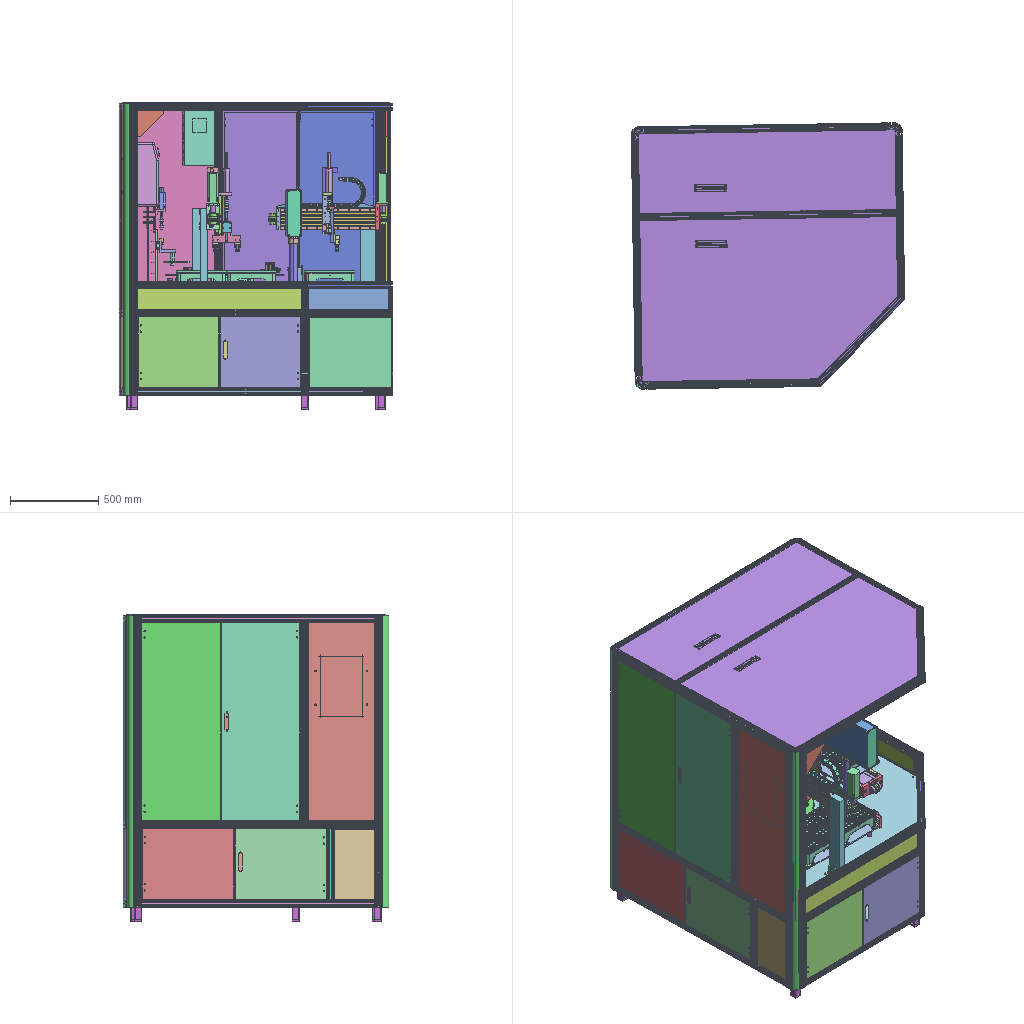Assembly | SolidWorks | 176 different items | 401 placed | box 1545 x 1502 x 1731 mm
Parts list (item | name | quantity | parent item):
1 | 12X20带轮  | x8 | in 25, 41, 57, 58
2 | 15x15×495导轨700 | x2 | in 69
3 | 15×15×186.5导轨 | x2 | in 25, 41
4 | 15×15×540导轨 | x4 | in 25, 41
5 | 4040角件 | x9 | in 25, 41, 91
6 | 4080型材 | x4 | in 25, 41
7 | 40X120型材 | x2 | in 25, 41
8 | 40X160型材 | x2 | in 57, 58
9 | 40×40×170型材(默认_按加工_) | x2 | in 10, 11
10 | 40×40×170型材（附端盖）-1 (subassembly) | x1 | in 82
11 | 40×40×170型材（附端盖） (subassembly) | x1 | in 82
12 | 40×40×250型材(默认_按加工_) | x1 | in 91
13 | 40型材端盖ARC52-4010-H4040 | x5 | in 10, 11, 91
14 | 80DF+0.55KW普通电机+050减速机(2018-5-28) (subassembly) | x1 | in 21
15 | 80x40×910铝型材 | x1 | in 69
16 | CDM2B20-100Z-XC8B双杆双作用气缸 | x2 | in 25, 41
17 | DNCJ 32X35-20-PPV-A气缸 | x1 | in 69
18 | DNCJ 32X60-20-PPV-A气缸 | x1 | in 69
19 | ECMA-C20604RS带刹车带油封 | x2 | in 25, 41
20 | HL-A-KDFJ-01 机架组件 (subassembly) | x1 | -
21 | HL-A-KDFJ-02 工作台机构 (subassembly) | x1 | -
22 | HL-A-KDFJ-02.1 圆盘 | x1 | in 21
23 | HL-A-KDFJ-02.2 分割器位置检测开关固定架 | x1 | in 21
24 | HL-A-KDFJ-02.3-1 分割器位置检测开关支架(Default) | x1 | in 21
25 | HL-A-KDFJ-03 抓取机构1 (subassembly) | x1 | -
26 | HL-A-KDFJ-03.1-1 带轮固定板 | x1 | in 25
27 | HL-A-KDFJ-03.1-2 带轮固定板2 | x1 | in 25
28 | HL-A-KDFJ-03.2-1 夹爪 | x4 | in 25
29 | HL-A-KDFJ-03.2-2 夹爪橡胶套 | x4 | in 25
30 | HL-A-KDFJ-03.2-3 气缸固定架 | x1 | in 25
31 | HL-A-KDFJ-03.2-4 抓取部件 | x1 | in 25
32 | HL-A-KDFJ-03.2-5 抓取部件1 | x1 | in 25
33 | HL-A-KDFJ-03.2-6 导轨固定架 | x1 | in 25
34 | HL-A-KDFJ-03.3-1.1 12×65轴 | x1 | in 25
35 | HL-A-KDFJ-03.3-1.1 12×80轴 | x1 | in 25
36 | HL-A-KDFJ-03.4-1 卸料链支架(默认) | x1 | in 25
37 | HL-A-KDFJ-03.4-2 拖链放置架 | x1 | in 25
38 | HL-A-KDFJ-03.5-1 导向块 | x1 | in 25
39 | HL-A-KDFJ-03.5-2 固定块 | x1 | in 25
40 | HL-A-KDFJ-03.6 压皮带块 | x2 | in 25
41 | HL-A-KDFJ-04 抓取机构2 (subassembly) | x1 | -
42 | HL-A-KDFJ-04.1 带轮固定板1 | x1 | in 41
43 | HL-A-KDFJ-04.2 带轮固定板2 | x1 | in 41
44 | HL-A-KDFJ-04.2-1 夹爪 | x4 | in 41
45 | HL-A-KDFJ-04.2-2 夹爪橡胶套 | x4 | in 41
46 | HL-A-KDFJ-04.2-3 气缸固定架 | x1 | in 41
47 | HL-A-KDFJ-04.2-4 抓取部件 | x1 | in 41
48 | HL-A-KDFJ-04.2-5 抓取部件1 | x1 | in 41
49 | HL-A-KDFJ-04.2-6 导轨固定架 | x1 | in 41
50 | HL-A-KDFJ-04.3-1.1 12×65轴  | x1 | in 41
51 | HL-A-KDFJ-04.3-1.1 12×80轴  | x1 | in 41
52 | HL-A-KDFJ-04.4-1 拖链放置架 | x1 | in 41
53 | HL-A-KDFJ-04.4-2 卸料链支架2(默认) | x1 | in 41
54 | HL-A-KDFJ-04.5-1 导向块 | x1 | in 41
55 | HL-A-KDFJ-04.5-2 固定块 | x1 | in 41
56 | HL-A-KDFJ-04.6 压皮带块 | x2 | in 41
57 | HL-A-KDFJ-05 直线模组装配-1 (subassembly) | x1 | -
58 | HL-A-KDFJ-05 直线模组装配 (subassembly) | x1 | -
59 | HL-A-KDFJ-05.1-1 带轮固定板 | x2 | in 57, 58
60 | HL-A-KDFJ-05.1-2 带轮固定板1 | x2 | in 57, 58
61 | HL-A-KDFJ-05.1-3 运动板 | x2 | in 57, 58
62 | HL-A-KDFJ-05.1-4 限位块 | x8 | in 57, 58
63 | HL-A-KDFJ-05.1-5 支撑柱 | x8 | in 57, 58
64 | HL-A-KDFJ-05.1-6 限位块2 | x4 | in 57, 58
65 | HL-A-KDFJ-05.2-1.1 12×65轴 (1) | x2 | in 57, 58
66 | HL-A-KDFJ-05.2-1.2 12×80轴 (2) | x2 | in 57, 58
67 | HL-A-KDFJ-05.3-1 压皮带块 | x4 | in 57, 58
68 | HL-A-KDFJ-05.3-2 带轮压紧块 | x2 | in 57, 58
69 | HL-A-KDFJ-06 检测跳火工装 (subassembly) | x1 | -
70 | HL-A-KDFJ-06.2-1 滑块支座 | x2 | in 69
71 | HL-A-KDFJ-06.2-2 尼龙棒 | x2 | in 69
72 | HL-A-KDFJ-06.2-3 气缸垫块 | x2 | in 69
73 | HL-A-KDFJ-06.2-4 油槽托架 | x2 | in 69
74 | HL-A-KDFJ-06.2-5 支撑架1 | x1 | in 69
75 | HL-A-KDFJ-06.2-6 支撑架 | x1 | in 69
76 | HL-A-KDFJ-06.3-1 电极头 | x8 | in 69
77 | HL-A-KDFJ-06.3-2 80针 | x8 | in 69
78 | HL-A-KDFJ-06.3-3 电极座 | x8 | in 69
79 | HL-A-KDFJ-06.3-4电极头触点 | x2 | in 69
80 | HL-A-KDFJ-06.5 三针绝缘板 | x1 | in 69
81 | HL-A-KDFJ-06.6 油杯 | x4 | in 69
82 | HL-A-KDFJ-07 高压包电柜组件 (subassembly) | x1 | -
83 | HL-A-KDFJ-07.1 高压包电柜 (subassembly) | x1 | in 82
84 | HL-A-KDFJ-07.1-1 包电柜右门(默认) | x1 | in 83
85 | HL-A-KDFJ-07.1-2 包电柜左门(默认) | x1 | in 83
86 | HL-A-KDFJ-07.1-3 包电柜柜体(默认) | x1 | in 83
87 | HL-A-KDFJ-08 吹气组件 (subassembly) | x1 | -
88 | HL-A-KDFJ-08.1-1 吹油架 | x1 | in 87
89 | HL-A-KDFJ-08.1-2 吹油气缸架 | x1 | in 87
90 | HL-A-KDFJ-08.2 吹气件 | x2 | in 87
91 | HL-A-KDFJ-09 位置检测机构 (subassembly) | x1 | -
92 | HL-A-KDFJ-09.1 行程开关固定钣金(默认) | x1 | in 91
93 | HL-A-KDFJ-10 毛刷机构 (subassembly) | x1 | -
94 | HL-A-KDFJ-10.1 毛刷托盘(默认) | x1 | in 93
95 | HL-A-KDFJ-10.2 去油毛刷支架 | x4 | in 93
96 | HL-A-KDFJ-11 卸料板 | x1 | -
97 | HL-A-KDFJ-12 检测开关安装架 | x2 | -
98 | MHZ2-20D-M9BW气缸 _ | x4 | in 25, 41
99 | SLD60-88步进电机 | x2 | in 57, 58
100 | YBLX-ME_8169行程开关 | x3 | in 91
101 | _X2_5B9E4F53_X0_1 | x1 | in 14
102 | _X2_5B9E4F53_X0_2 | x1 | in 14
103 | _X2_5B9E4F53_X0_3 | x1 | in 14
104 | _X2_5B9E4F53_X0_4 | x1 | in 14
105 | 伺服电机联轴器 | x2 | in 25, 41
106 | 储物柜(默认) | x1 | in 20
107 | 储物柜门右(默认) | x1 | in 20
108 | 储物柜门左(默认) | x1 | in 20
109 | 分割器感应开关 | x1 | in 21
110 | 右侧电器板 | x1 | in 20
111 | 右电气柜(默认) | x1 | in 20
112 | 型材角码 | x9 | in 25, 41, 69
113 | 复件  | x2 | in 20
114 | - | x6 | in 20
115 | - | x1 | in 160
116 | - | x1 | in 160
117 | - | x1 | in 160
118 | - | x1 | in 160
119 | - | x1 | in 160
120 | - | x2 | in 160
121 | - | x1 | in 160
122 | - | x2 | in 160
123 | 复件 _VBD32-F25-R75-N17-001^拖链VBD32-F25-R75-N17 | x34 | in 152, 153
124 | 复件 _VED32-F25-001^拖链VBD32-F25-R75-N17 | x2 | in 152, 153
125 | 复件 _VED32-F25-002^拖链VBD32-F25-R75-N17 | x2 | in 152, 153
126 | - | x1 | in 20
127 | - | x2 | in 160
128 | - | x1 | in 160
129 | 复件 复件 (10)  | x2 | in 20
130 | 复件 复件 (11)  | x1 | in 20
131 | 复件 复件 (13)  | x1 | in 20
132 | 复件 复件 (14)  | x1 | in 20
133 | 复件 复件 (15)  | x1 | in 20
134 | 复件 复件 (16)  | x1 | in 20
135 | 复件 复件 (17)  | x3 | in 20
136 | 复件 复件 (2)  | x2 | in 20
137 | 复件 复件 (3)  | x1 | in 20
138 | 复件 复件 (4)  | x2 | in 20
139 | 复件 复件 (5)  | x3 | in 20
140 | 复件 复件 (6)  | x3 | in 20
141 | 复件 复件 (7)  | x2 | in 20
142 | 复件 复件 (8)  | x2 | in 20
143 | 复件 复件 (9)  | x2 | in 20
144 | 导轨700 | x4 | in 57, 58
145 | 封闭柜体(默认) | x1 | in 20
146 | 工作台大板 | x1 | in 20
147 | 左侧电器板 | x1 | in 20
148 | 左电气柜(默认) | x1 | in 20
149 | 带座轴承 | x8 | in 25, 41
150 | 悬挂油箱 | x1 | -
151 | 悬挂油箱背板(默认) | x1 | in 20
152 | 拖链VBD32-F25-R75-N17-1 (subassembly) | x1 | in 41
153 | 拖链VBD32-F25-R75-N17 (subassembly) | x1 | in 25
154 | 显示器立柱 | x1 | -
155 | 机架右侧门(默认) | x1 | in 20
156 | 机架右侧门2(默认) | x1 | in 20
157 | 机架后侧门(默认) | x1 | in 20
158 | 机架后侧门2(默认) | x1 | in 20
159 | 模具 | x4 | -
160 | 气缸20x30 (subassembly) | x1 | in 87
161 | 油箱 | x1 | in 20
162 | 油箱侧柜门右(默认) | x1 | in 20
163 | 油箱侧柜门左(默认) | x1 | in 20
164 | 油箱门右(默认) | x1 | in 20
165 | 油箱门左(默认) | x1 | in 20
166 | 滑块 | x16 | in 25, 41, 57, 58, 69
167 | 焊接板 | x1 | in 20
168 | 电器柜门左(默认) | x1 | in 20
169 | 电气柜门右(默认) | x1 | in 20
170 | 盖板(默认) | x1 | in 20
171 | 立式KP001轴承套2 | x8 | in 57, 58
172 | 联轴器8X12 | x2 | in 57, 58
173 | 角撑 | x2 | in 20
174 | 角码 | x8 | in 25, 41
175 | 转接头 | x5 | in 25, 41, 69
176 | 零件1 | x1 | in 20